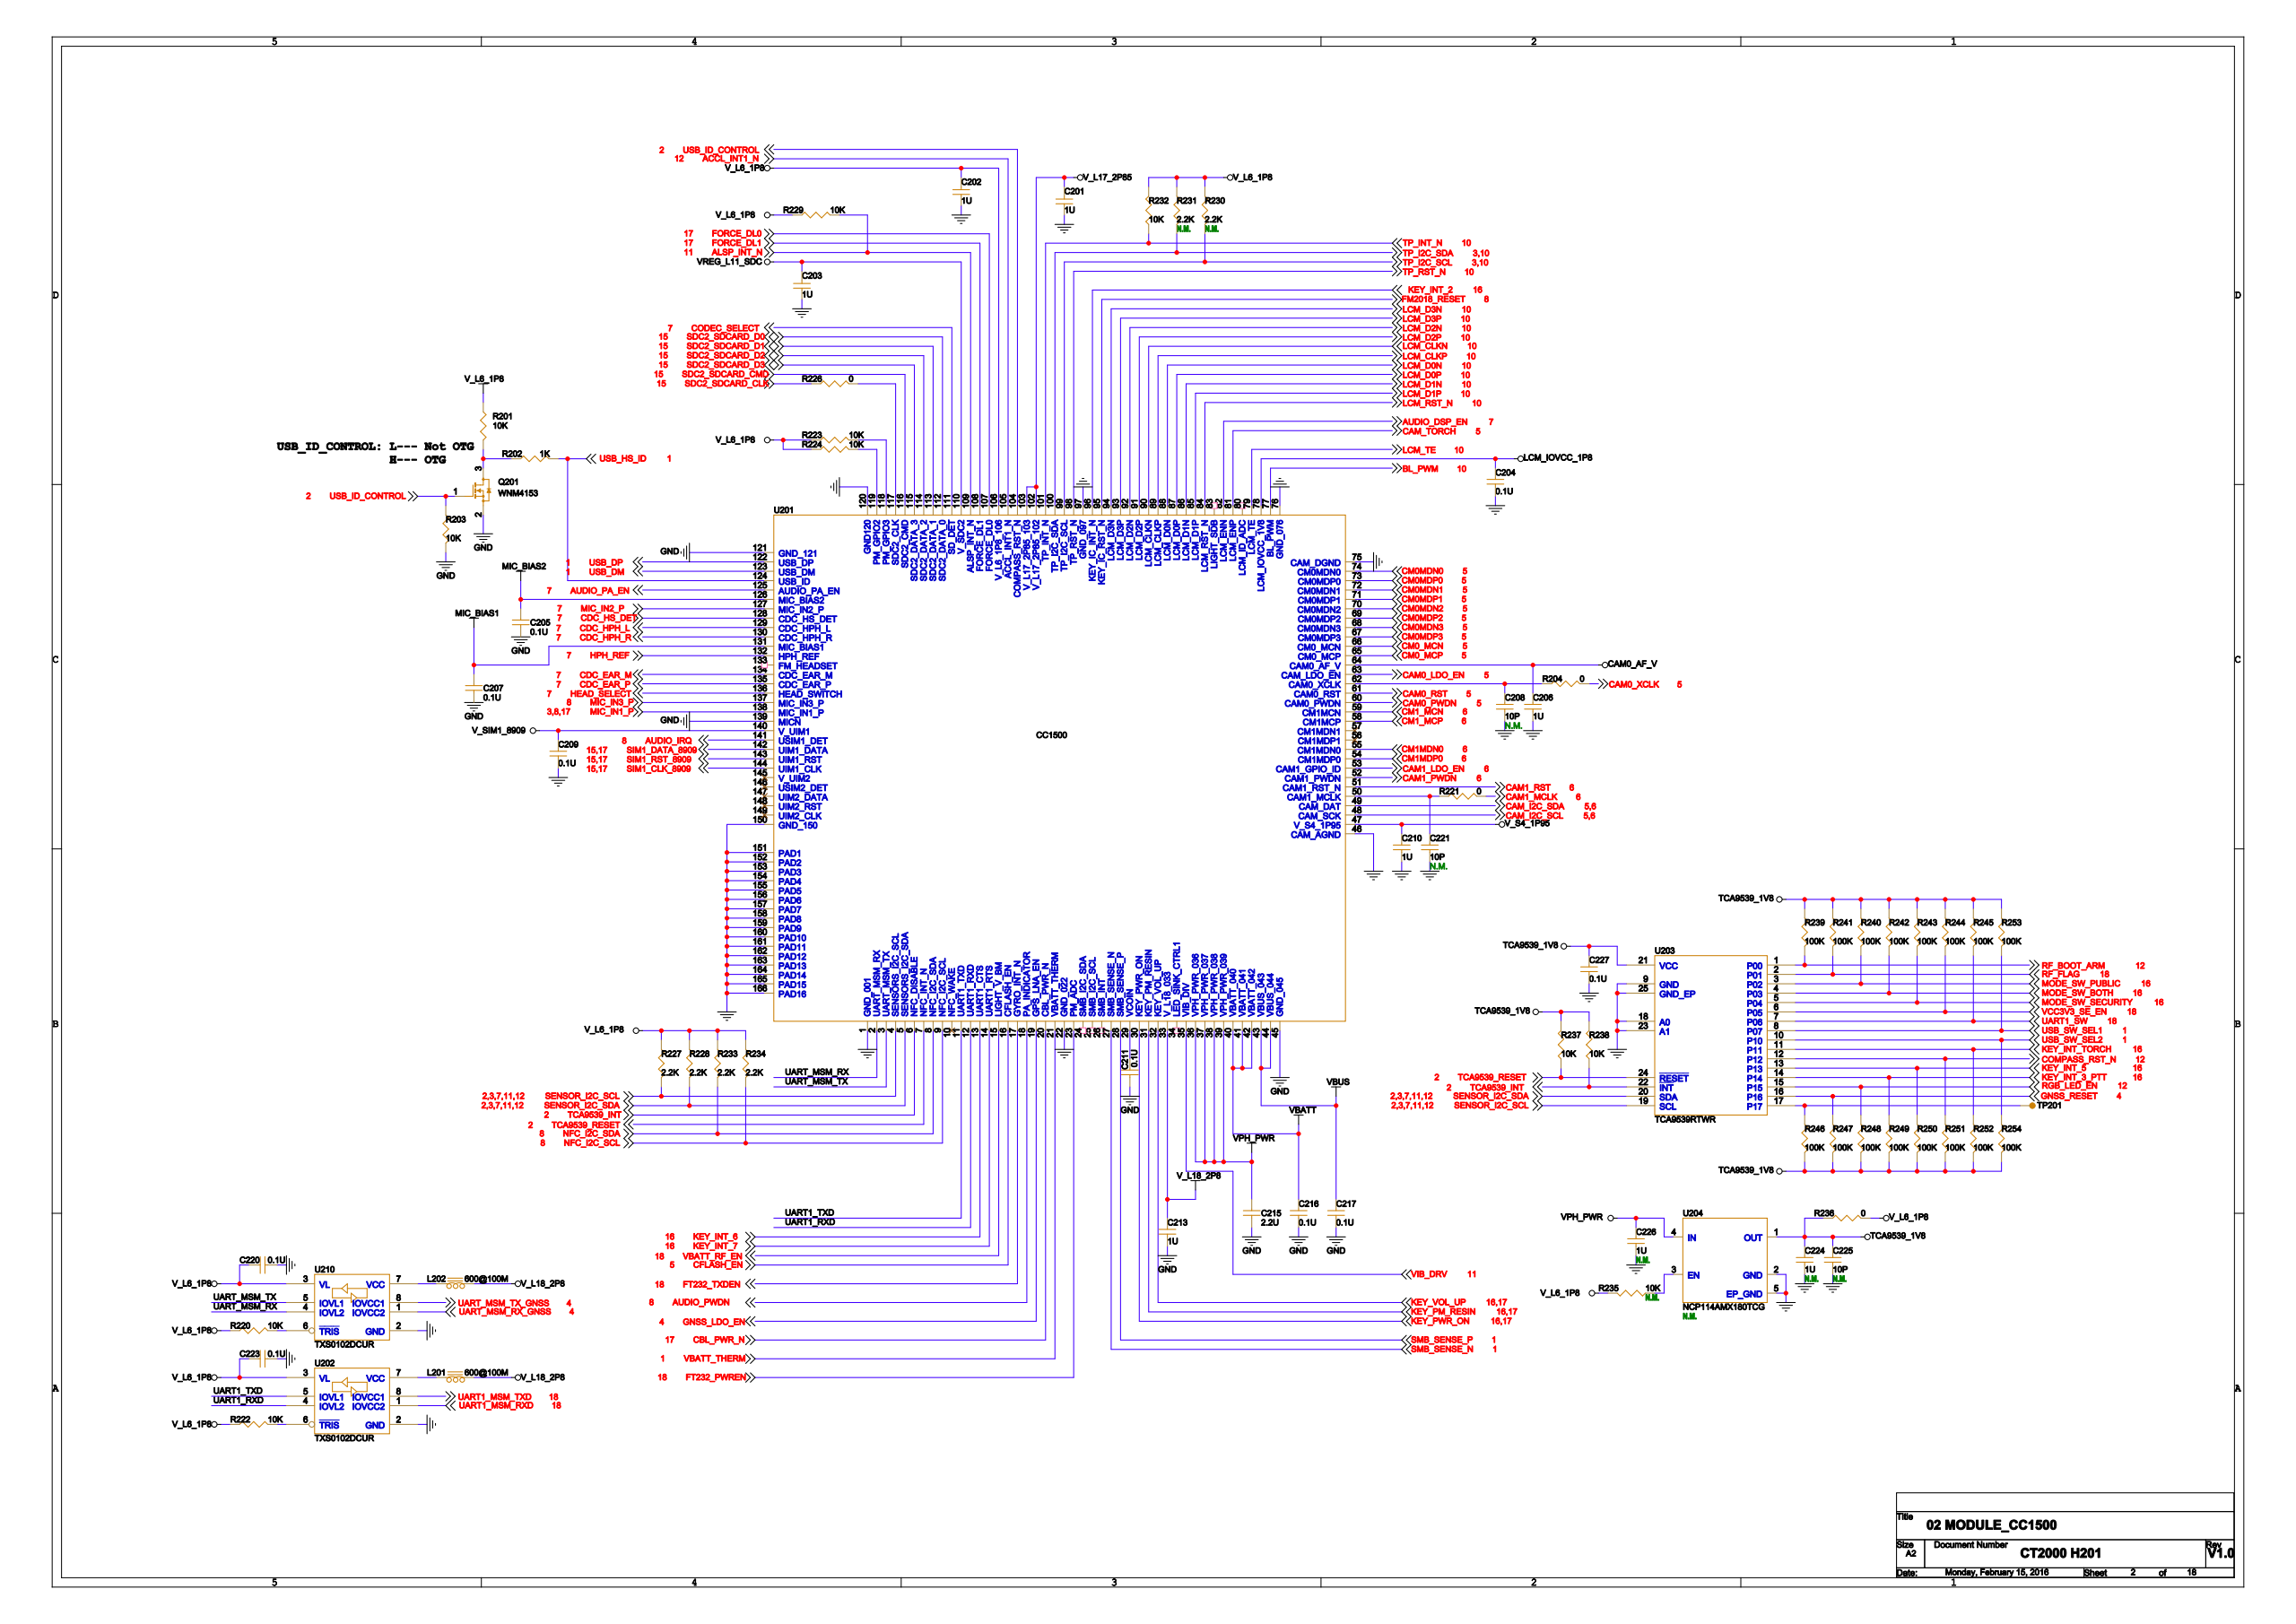Circuit board | Cadence Allegro | 573 parts | 376 nets | one sheet of the schematic
Parts on this sheet (reference | value | footprint):
C201 | 1U | C0402
C202 | 1U | C0402
C203 | 1U | C0402
C204 | 0.1U | C0402
C205 | 0.1U | C0402
C206 | 1U | C0402
C207 | 0.1U | C0402
C208 | 10P | C0402
C209 | 0.1U | C0402
C210 | 1U | C0402
C211 | 0.1U | C0402
C213 | 1U | C0402
C215 | 2.2U | C0402
C216 | 0.1U | C0402
C217 | 0.1U | C0402
C220 | 0.1U | C0402
C221 | 10P | C0402
C224 | 1U | C0402
C225 | 10P | C0402
C226 | 1U | C0402
C227 | 0.1U | C0402
L202 | 600@100M | L0402
Q201 | WNM4153 | SOT-523
R201 | 10K | R0402
R202 | 1K | R0402
R203 | 10K | R0402
R204 | 0 | R0402
R220 | 10K | R0402
R221 | 0 | R0402
R223 | 10K | R0402
R224 | 10K | R0402
R226 | 0 | R0402
R227 | 2.2K | R0402
R228 | 2.2K | R0402
R229 | 10K | R0402
R230 | 2.2K | R0402
R231 | 2.2K | R0402
R232 | 10K | R0402
R233 | 2.2K | R0402
R234 | 2.2K | R0402
R235 | 10K | R0402
R236 | 0 | R0402
R237 | 10K | R0402
R238 | 10K | R0402
R239 | 100K | R0402
R240 | 100K | R0402
R241 | 100K | R0402
R242 | 100K | R0402
R243 | 100K | R0402
R244 | 100K | R0402
R245 | 100K | R0402
R246 | 100K | R0402
R247 | 100K | R0402
R248 | 100K | R0402
R249 | 100K | R0402
R250 | 100K | R0402
R251 | 100K | R0402
R252 | 100K | R0402
R253 | 100K | R0402
R254 | 100K | R0402
TP201 | 1 mm | TESTPOINT_32MIL
U201 | CC1500 | MODULE_CC1500
U203 | TCA9539RTWR | QFN24_4X4X0P9_0P5
U204 | NCP114AMX180TCG | UDFN4_1X1X0P7_0P65
U210 | TXS0102DCUR | SOT-70
Nets of these parts (net: part-pin ...):
GND: C201-1 C202-1 C203-1 C204-2 C205-2 C206-2 C207-2 C208-2 C209-2 C210-2 C211-2 C213-2 C215-2 C216-2 C217-2 C220-2 C221-2 C224-2 C225-2 C226-2 C227-2 Q201-2 R203-2 U204-2 U204-5 U210-2 U201-1 U201-22 U201-45 U201-46 U201-75 U201-76 U201-97 U201-120 U201-121 U201-139 U201-150 U201-151 U201-152 U201-153 U201-154 U201-155 U201-156 U201-157 U201-158 U201-159 U201-160 U201-161 U201-162 U201-163 U201-164 U201-165 U201-166 U203-9 U203-18 U203-23 U203-25
UART_MSM_TX_GNSS: U210-8
UART_MSM_RX_GNSS: U210-1
FT232_TXDEN: U201-17
FT232_PWREN: U201-23
MIC_IN1_P: U201-138
LCM_TE: U201-79
LCM_IOVCC_1P8: C204-1 U201-78
TP_I2C_SDA: R231-2 U201-100
TP_I2C_SCL: R230-2 U201-99
TP_RST_N: U201-98
TP_INT_N: R232-2 U201-101
KEY_INT_3_PTT: R249-2 U203-14
KEY_PM_RESIN: U201-31
KEY_VOL_UP: U201-32
KEY_INT_7: U201-14
KEY_INT_6: U201-13
KEY_INT_5: R250-2 U203-13
VBATT: C216-1 U201-40 U201-41 U201-42
MIC_BIAS1: C207-1 U201-131
ALSP_INT_N: R229-1 U201-109
SENSOR_I2C_SDA: R228-2 U201-5 U203-20
V_L17_2P85: C201-2 U201-102 U201-103
VPH_PWR: C215-1 C226-1 U204-4 U201-36 U201-37 U201-38 U201-39
SENSOR_I2C_SCL: R227-2 U201-4 U203-19
SDC2_SDCARD_CMD: U201-116
KEY_INT_2: U201-96
KEY_INT_TORCH: R252-2 U203-11
KEY_PWR_ON: U201-30
V_SIM1_8909: C209-1 U201-140
MODE_SW_PUBLIC: R240-1 U203-3
MODE_SW_BOTH: R242-1 U203-4
MODE_SW_SECURITY: R243-1 U203-5
USB_DP: U201-122
USB_DM: U201-123
VBUS: C217-1 U201-43 U201-44
N52714154: R235-2 U204-3
TCA9539_1V8: C224-1 C225-1 C227-1 R236-1 R237-1 R238-1 R239-2 R240-2 R241-2 R242-2 R243-2 R244-2 R245-2 R246-1 R247-1 R248-1 R249-1 R250-1 R251-1 R252-1 R253-2 R254-1 U204-1 U203-21
CAM0_LDO_EN: U201-63
CAM1_LDO_EN: U201-53
AUDIO_DSP_EN: U201-82
ACCL_INT1_N: U201-105
AUDIO_PA_EN: U201-125
BL_PWM: U201-77
CAM0_AF_V: C206-1 U201-64
CAM0_PWDN: U201-60
CAM0_RST: U201-61
N51849529: C208-1 R204-1 U201-62
N52175112: C221-1 R221-1 U201-50
CAM1_PWDN: U201-52
CAM1_RST: U201-51
CAM_I2C_SDA: U201-49
CAM_I2C_SCL: U201-48
CBL_PWR_N: U201-20
CDC_EAR_M: U201-134
CDC_EAR_P: U201-135
CDC_HPH_L: U201-129
CDC_HPH_R: U201-130
CDC_HS_DET: U201-128
CFLASH_EN: U201-16
CM0MDN0: U201-74
CM0MDN1: U201-72
CM0MDN2: U201-70
CM0MDN3: U201-68
CM0MDP0: U201-73
CM0MDP1: U201-71
CM0MDP2: U201-69
CM0MDP3: U201-67
CM0_MCN: U201-66
CM0_MCP: U201-65
CM1_MCN: U201-59
CM1_MCP: U201-58
CM1MDN0: U201-55
CM1MDP0: U201-54
USB_ID_CONTROL: Q201-1 R203-1 U201-104
FORCE_DL0: U201-107
FORCE_DL1: U201-108
GNSS_LDO_EN: U201-19
HEAD_SELECT: U201-136
HPH_REF: U201-132
FM2018_RESET: U201-95
LCM_CLKN: U201-90
LCM_CLKP: U201-89
LCM_D0N: U201-88
LCM_D0P: U201-87
LCM_D1N: U201-86
LCM_D1P: U201-85
LCM_D2N: U201-92
LCM_D2P: U201-91
LCM_D3N: U201-94
LCM_D3P: U201-93
CAM_TORCH: U201-81
LCM_RST_N: U201-84
VBATT_RF_EN: U201-15
MIC_BIAS2: C205-1 U201-126
MIC_IN2_P: U201-127
MIC_IN3_P: U201-137
TCA9539_INT: R238-2 U201-6 U203-22
NFC_I2C_SCL: R234-2 U201-9
NFC_I2C_SDA: R233-2 U201-8
TCA9539_RESET: R237-2 U201-7 U203-24
AUDIO_PWDN: U201-18
N52251706: R224-1 U201-119
N52251713: R223-1 U201-118
N52251896: R226-2 U201-117
SDC2_SDCARD_D0: U201-112
SDC2_SDCARD_D1: U201-113
SDC2_SDCARD_D2: U201-114
SDC2_SDCARD_D3: U201-115
CODEC_SELECT: U201-111
SMB_SENSE_N: U201-27
SMB_SENSE_P: U201-28
UART1_MSM_RXD: U201-12
UART1_MSM_TXD: U201-11
UART_MSM_RX: U210-4 U201-2
UART_MSM_TX: U210-5 U201-3
SIM1_CLK_8909: U201-144
SIM1_DATA_8909: U201-142
SIM1_RST_8909: U201-143
USB_HS_ID: R202-2 U201-124
AUDIO_IRQ: U201-141
VBATT_THERM: U201-21
N51842021: C211-1 U201-29
VIB_DRV: U201-35
V_L18_2P8: C213-1 L202-2 U201-33
V_L6_1P8: C202-2 C220-1 R201-1 R220-1 R223-2 R224-2 R227-1 R228-1 R229-2 R230-1 R231-1 R232-1 R233-1 R234-1 R235-1 R236-2 U210-3 U201-106
V_S4_1P95: C210-1 U201-47
VREG_L11_SDC: C203-2 U201-110
RF_BOOT_ARM: R239-1 U203-1
RF_FLAG: R241-1 U203-2
VCC3V3_SE_EN: R244-1 U203-6
UART1_SW: R245-1 U203-7
USB_SW_SEL1: R253-1 U203-8
USB_SW_SEL2: R254-2 U203-10
COMPASS_RST_N: R251-2 U203-12
RGB_LED_EN: R248-2 U203-15
GNSS_RESET: R247-2 U203-16
N52719549: R246-2 TP201-1 U203-17
CAM1_MCLK: R221-2
CAM0_XCLK: R204-2
SDC2_SDCARD_CLK: R226-1
N52086250: L202-1 U210-7
N51882747: Q201-3 R201-2 R202-1
N52086268: R220-2 U210-6